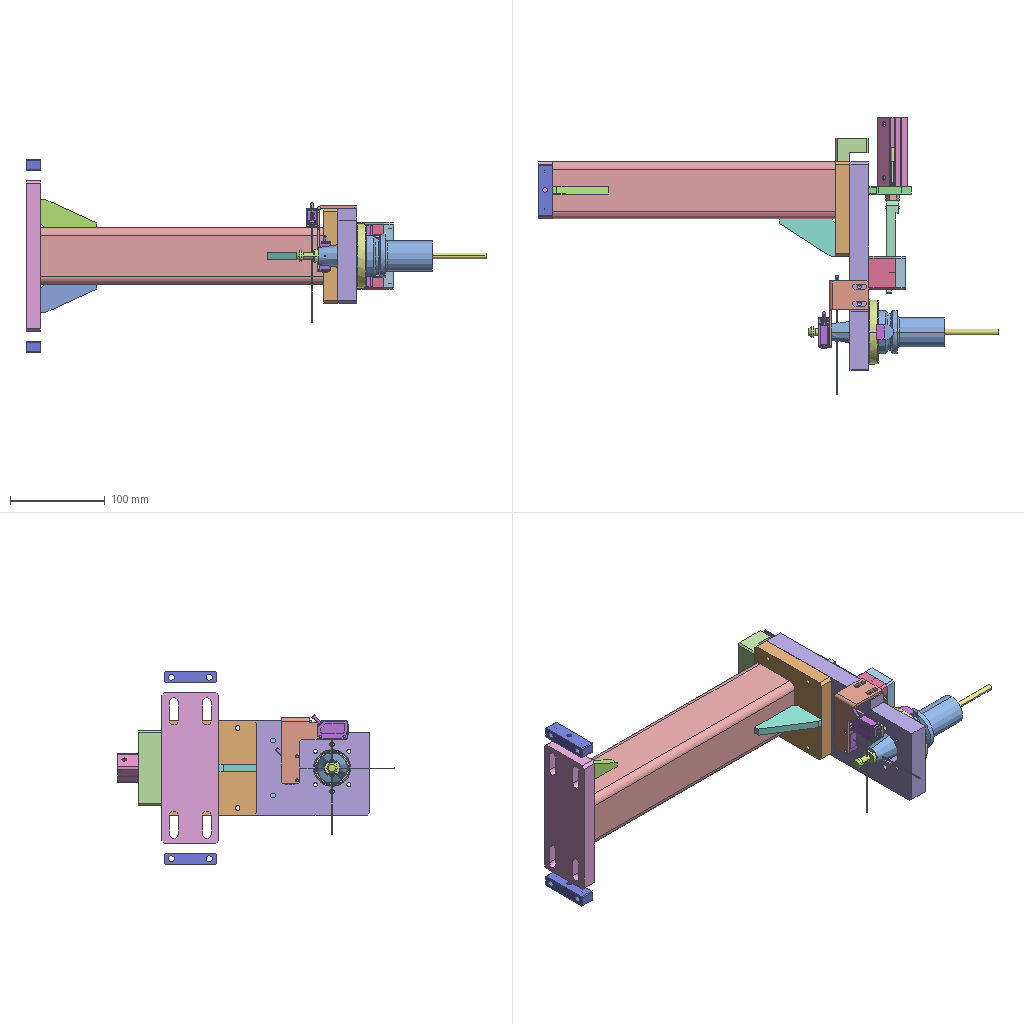Assembly | SolidWorks | 15 different items | 18 placed | box 487 x 293 x 204 mm
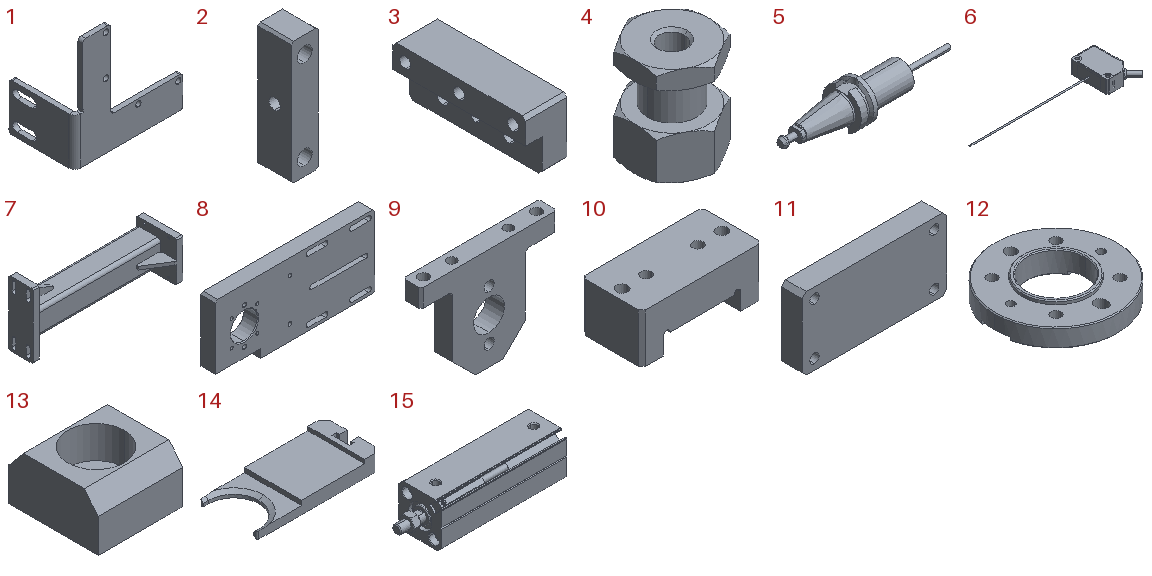Parts list (item | quantity | size | volume | features):
1 | x1 | 69 x 42 x 70 mm | 9835 mm3 | features HoleWzd 2, EdgeFlange 1, Fillet 1, FlatPattern 1, SMBaseFlange 1, SheetMetal 1
2 | x2 | 12 x 15 x 55 mm | 7635 mm3 | features HoleWzd 2, Chamfer 1, Extrusion 1
3 | x1 | 25 x 80 x 35 mm | 46243 mm3 | features HoleWzd 3, Chamfer 1, Extrusion 1
4 | x1 | 12 x 13.856 x 16 mm | 1324 mm3 | features BaseBody 1
5 | x1 | 200 x 46 x 46 mm | 92799 mm3 | features BaseBody 10, MoveFace 1
6 | x2 | - | - | features BaseBody 1, ExtruRefSurface 1
7 | x1 | 330 x 100 x 160 mm | 561297 mm3 | features HoleWzd 4, ICE 4, Chamfer 2, MirrorSolid 1, WeldMemberFeat 1, WeldmentFeature 1
8 | x1 | 220 x 20 x 100 mm | 365463 mm3 | features HoleWzd 11, Chamfer 2, ICE 2, Cut 1, Extrusion 1
9 | x1 | 60 x 8 x 45 mm | 10317 mm3 | features HoleWzd 3, Chamfer 2, Extrusion 1, ICE 1
10 | x1 | 70 x 35 x 28.4 mm | 48866 mm3 | features HoleWzd 3, Chamfer 1, Extrusion 1, ICE 1
11 | x1 | 70 x 10 x 35 mm | 23097 mm3 | features Chamfer 1, Extrusion 1, HoleWzd 1
12 | x1 | 68 x 68 x 12 mm | 24199 mm3 | features HoleWzd 4, Chamfer 1, ICE 1, Revolution 1
13 | x2 | 15 x 15.8 x 9 mm | 1494 mm3 | features Extrusion 1, HoleWzd 1, ICE 1
14 | x1 | 98 x 45 x 13 mm | 33070 mm3 | features Chamfer 5, ICE 4, Fillet 2, Cavity 1, Cut 1, Extrusion 1
15 | x1 | 87 x 25 x 25 mm | 36793 mm3 | features BaseBody 5, MoveCopyBody 2
Mates (type | each side: item.copy, entity, surface, feature):
Coincident | 7.1 face plane Boss-Extrude 3 | 8.1 face plane Boss-Extrude 1 | 2 times
Width | 8.1 face plane Boss-Extrude 1 | 8.1 face plane Boss-Extrude 1 | 7.1 face plane Boss-Extrude 3 | 7.1 face plane Boss-Extrude 3
Coincident | 8.1 face plane Boss-Extrude 1 | 9.1 face plane Boss-Extrude 1
Concentric | 8.1 face cylinder Ø4.0mm 暗销Hole 1 | 9.1 face cylinder Ø4.0mm 暗销Hole 1
Coincident | 8.1 face cylinder Ø4.0mm 暗销Hole 1 | 9.1 edge
Coincident | 9.1 face plane Boss-Extrude 1 | 15.1 face plane _ACQS-12x4545_b-1-solid1
Concentric | 9.1 face cylinder Cut-Extrude 1 | 15.1 face cylinder _ACQS-12x4545_b-1-solid1
Concentric | 9.1 face cylinder M4 六角圆柱头Screw的柱形沉头Hole 2 | 15.1 face cylinder _ACQS-12x4545_b-1-solid1
Coincident | 8.1 face plane Boss-Extrude 1 | 10.1 face plane Boss-Extrude 1
Concentric | 8.1 face cylinder Ø6.0mm 暗销Hole 1 | 10.1 face cylinder Ø6.0mm 暗销Hole 1 | 2 times
Coincident | 10.1 face plane Boss-Extrude 1 | 11.1 face plane Boss-Extrude 1
Concentric | 10.1 face cylinder M4 Tapped Hole 1 | 11.1 face cylinder M4 六角圆柱头Screw的柱形沉头Hole 1 | 2 times
Concentric | 8.1 face cylinder Cut-Extrude 2 | 12.1 face cylinder Revolve 1
Coincident | 8.1 face plane Boss-Extrude 1 | 12.1 face plane Revolve 1
Concentric | 8.1 face cylinder Ø6.0mm 暗销Hole 2 | 12.1 face cylinder Ø6.0mm 暗销Hole 1
Coincident | 12.1 face plane Cut-Extrude 1 | 13.1 face plane Boss-Extrude 1
Concentric | 12.1 face cylinder M5 Tapped Hole 1 | 13.1 face cylinder M4 沉头Hole 1
Parallel | 12.1 face plane Cut-Extrude 1 | 13.1 face plane Boss-Extrude 1
Coincident | 12.1 face plane Cut-Extrude 1 | 13.2 face plane Boss-Extrude 1
Concentric | 12.1 face cylinder M5 Tapped Hole 1 | 13.2 face cylinder M4 沉头Hole 1
Parallel | 12.1 face plane Cut-Extrude 1 | 13.2 face plane Boss-Extrude 1
Concentric | 12.1 face cylinder Revolve 1 | 5.1 face cylinder BT30刀柄-0725-1-solid1
Coincident | 12.1 face plane Revolve 1 | 5.1 face plane BT30刀柄-0725-1-solid1
Parallel | 13.1 face plane Boss-Extrude 1 | 5.1 face plane BT30刀柄-0725-1-solid1
Concentric | 15.1 face cylinder _ACQS-12x45-B_45r-1-solid1 | 4.1 face cylinder 输入1
Coincident | 15.1 face plane _ACQ 12_Nut-1-solid1 | 4.1 face plane 输入1
Coincident | 8.1 face plane Boss-Extrude 1 | 1.1 face plane Edge-Flange 1 | 2 times
Coincident | 1.1 face plane Base-Flange 1 | 6.1 face plane E-MSMD61N-2M_l-1-solid1
Concentric | 1.1 face cylinder M3 间隙Hole 1 | 6.1 face cylinder E-MSMD61N-2M_l-1-solid1 | 2 times
Coincident | 1.1 face plane Base-Flange 1 | 6.2 face plane E-MSMD61N-2M_l-1-solid1
Concentric | 1.1 face cylinder M3 间隙Hole 1 | 6.2 face cylinder E-MSMD61N-2M_l-1-solid1 | 2 times
Slot | 8.1 face cylinder M5 Tapped Hole 2 | 1.1 face plane M5 间隙槽口3
Coincident | 7.1 face plane Boss-Extrude 1 | 2.1 face plane Boss-Extrude 1
DistanceDim | 7.1 face plane Boss-Extrude 1 | 2.1 face plane Boss-Extrude 1
Width | 7.1 face plane Boss-Extrude 1 | 7.1 face plane Boss-Extrude 1 | 2.1 face plane Boss-Extrude 1 | 2.1 face plane Boss-Extrude 1
Coincident | 7.1 face plane Boss-Extrude 1 | 2.2 face plane Boss-Extrude 1
DistanceDim | 2.2 face plane Boss-Extrude 1 | 7.1 face plane Boss-Extrude 1
Coincident | 2.1 face plane Boss-Extrude 1 | 2.2 face plane Boss-Extrude 1
Coincident | 7.1 face plane Boss-Extrude 3 | 3.1 face plane Boss-Extrude 1
Concentric | 7.1 face cylinder M6 Tapped Hole 2 | 3.1 face cylinder M6 六角圆柱头Screw的柱形沉头Hole 1 | 2 times
Coincident | 10.1 face plane Boss-Extrude 1 | 14.1 face plane Boss-Extrude 1
Symmetric | 8.1 face plane Boss-Extrude 1 | 8.1 face plane Boss-Extrude 1 | 14.1 plane
Width | 14.1 face plane Boss-Extrude 1 | 14.1 face plane Cut-Extrude 2 | 4.1 face plane 输入1 | 4.1 face plane 输入1